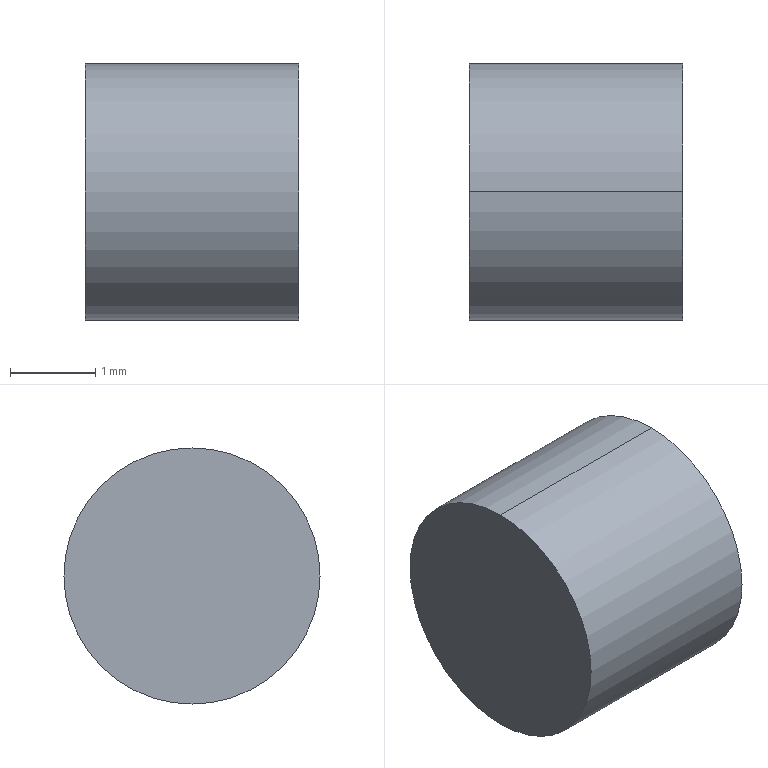Part | NX | features solid 2 | 1 solid | 4 faces | box 2.5 x 3 x 3 mm | volume 17.671 mm3 | plane 2 | cylinder 2 | commonest cylinder face diameters 3 x2
STEP:
#1=CARTESIAN_POINT('',(-297.5,938.55,-384.5));
#2=VERTEX_POINT('',#1);
#3=CARTESIAN_POINT('',(-297.5,938.55,-387.5));
#4=VERTEX_POINT('',#3);
#5=CARTESIAN_POINT('',(-297.5,938.55,-386.));
#6=DIRECTION('',(1.,0.,0.));
#7=DIRECTION('',(0.,0.,1.));
#8=AXIS2_PLACEMENT_3D('',#5,#6,#7);
#9=CIRCLE('',#8,1.5);
#10=EDGE_CURVE('',#2,#4,#9,.T.);
#11=ORIENTED_EDGE('',*,*,#10,.F.);
#12=CARTESIAN_POINT('',(-297.5,938.55,-386.));
#13=DIRECTION('',(1.,0.,0.));
#14=DIRECTION('',(0.,0.,-1.));
#15=AXIS2_PLACEMENT_3D('',#12,#13,#14);
#16=CIRCLE('',#15,1.5);
#17=EDGE_CURVE('',#4,#2,#16,.T.);
#18=ORIENTED_EDGE('',*,*,#17,.F.);
#19=EDGE_LOOP('',(#11,#18));
#20=FACE_BOUND('',#19,.T.);
#21=CARTESIAN_POINT('',(-297.5,938.55,-386.));
#22=DIRECTION('',(1.,0.,0.));
#23=DIRECTION('',(0.,0.,1.));
#24=AXIS2_PLACEMENT_3D('',#21,#22,#23);
#25=PLANE('',#24);
#26=ADVANCED_FACE('',(#20),#25,.F.);
#27=CARTESIAN_POINT('',(-295.,938.55,-384.5));
#28=VERTEX_POINT('',#27);
#29=CARTESIAN_POINT('',(-297.5,938.55,-384.5));
#30=DIRECTION('',(1.,0.,0.));
#31=VECTOR('',#30,1000.);
#32=LINE('',#29,#31);
#33=EDGE_CURVE('',#28,#2,#32,.F.);
#34=ORIENTED_EDGE('',*,*,#33,.F.);
#35=CARTESIAN_POINT('',(-295.,938.55,-387.5));
#36=VERTEX_POINT('',#35);
#37=CARTESIAN_POINT('',(-295.,938.55,-386.));
#38=DIRECTION('',(-1.,0.,0.));
#39=DIRECTION('',(0.,0.,1.));
#40=AXIS2_PLACEMENT_3D('',#37,#38,#39);
#41=CIRCLE('',#40,1.5);
#42=EDGE_CURVE('',#28,#36,#41,.T.);
#43=ORIENTED_EDGE('',*,*,#42,.T.);
#44=CARTESIAN_POINT('',(-297.5,938.55,-387.5));
#45=DIRECTION('',(1.,0.,0.));
#46=VECTOR('',#45,1000.);
#47=LINE('',#44,#46);
#48=EDGE_CURVE('',#4,#36,#47,.T.);
#49=ORIENTED_EDGE('',*,*,#48,.F.);
#50=ORIENTED_EDGE('',*,*,#17,.T.);
#51=EDGE_LOOP('',(#34,#43,#49,#50));
#52=FACE_BOUND('',#51,.T.);
#53=CARTESIAN_POINT('',(-297.5,938.55,-386.));
#54=DIRECTION('',(1.,0.,0.));
#55=DIRECTION('',(0.,0.,1.));
#56=AXIS2_PLACEMENT_3D('',#53,#54,#55);
#57=CYLINDRICAL_SURFACE('',#56,1.5);
#58=ADVANCED_FACE('',(#52),#57,.T.);
#59=ORIENTED_EDGE('',*,*,#48,.T.);
#60=CARTESIAN_POINT('',(-295.,938.55,-386.));
#61=DIRECTION('',(-1.,0.,0.));
#62=DIRECTION('',(0.,0.,-1.));
#63=AXIS2_PLACEMENT_3D('',#60,#61,#62);
#64=CIRCLE('',#63,1.5);
#65=EDGE_CURVE('',#36,#28,#64,.T.);
#66=ORIENTED_EDGE('',*,*,#65,.T.);
#67=ORIENTED_EDGE('',*,*,#33,.T.);
#68=ORIENTED_EDGE('',*,*,#10,.T.);
#69=EDGE_LOOP('',(#59,#66,#67,#68));
#70=FACE_BOUND('',#69,.T.);
#71=CARTESIAN_POINT('',(-297.5,938.55,-386.));
#72=DIRECTION('',(1.,0.,0.));
#73=DIRECTION('',(0.,0.,1.));
#74=AXIS2_PLACEMENT_3D('',#71,#72,#73);
#75=CYLINDRICAL_SURFACE('',#74,1.5);
#76=ADVANCED_FACE('',(#70),#75,.T.);
#77=ORIENTED_EDGE('',*,*,#65,.F.);
#78=ORIENTED_EDGE('',*,*,#42,.F.);
#79=EDGE_LOOP('',(#77,#78));
#80=FACE_BOUND('',#79,.T.);
#81=CARTESIAN_POINT('',(-295.,938.55,-386.));
#82=DIRECTION('',(1.,0.,0.));
#83=DIRECTION('',(0.,0.,1.));
#84=AXIS2_PLACEMENT_3D('',#81,#82,#83);
#85=PLANE('',#84);
#86=ADVANCED_FACE('',(#80),#85,.T.);
#87=CLOSED_SHELL('',(#26,#58,#76,#86));
#88=MANIFOLD_SOLID_BREP('',#87);
#89=(LENGTH_UNIT()NAMED_UNIT(*)SI_UNIT(.MILLI.,.METRE.));
#90=UNCERTAINTY_MEASURE_WITH_UNIT(LENGTH_MEASURE(0.00001),#89,'','');
#91=(NAMED_UNIT(*)PLANE_ANGLE_UNIT()SI_UNIT($,.RADIAN.));
#92=(NAMED_UNIT(*)SI_UNIT($,.STERADIAN.)SOLID_ANGLE_UNIT());
#93=(GEOMETRIC_REPRESENTATION_CONTEXT(3)GLOBAL_UNCERTAINTY_ASSIGNED_CONTEXT((#90))GLOBAL_UNIT_ASSIGNED_CONTEXT((#89,#91,#92))REPRESENTATION_CONTEXT('',''));
#94=ADVANCED_BREP_SHAPE_REPRESENTATION('',(#88),#93);